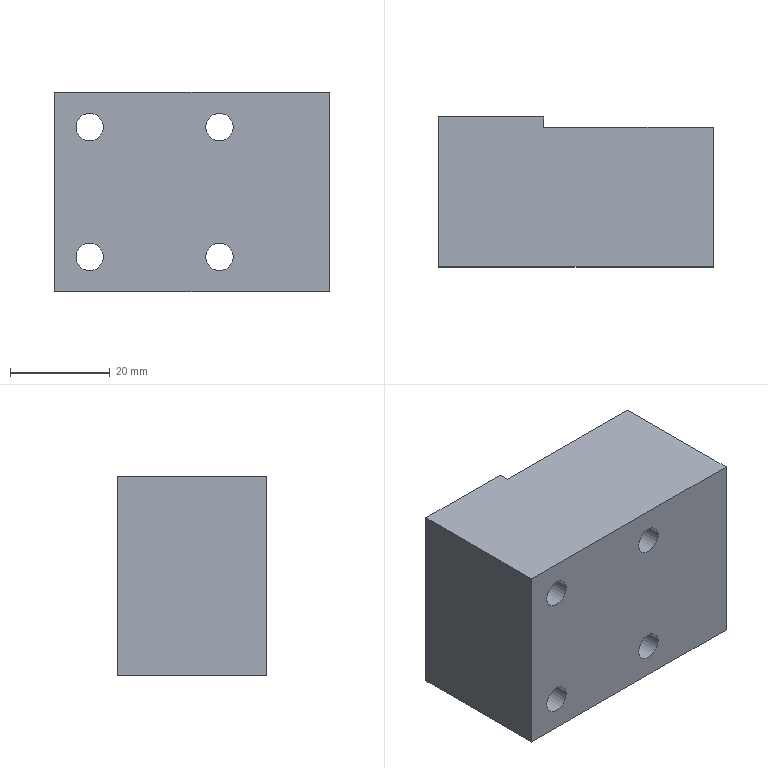Part | NX | features BREP 1 | 1 solid | 24 faces | box 55 x 30 x 40 mm | volume 57495 mm3 | plane 12 | cylinder 10 | cone 2 | commonest cylinder face diameters 5.5 x4 10 x4 6.8 x2
STEP:
#1=CARTESIAN_POINT('',(7.,30.,18.));
#2=VERTEX_POINT('',#1);
#3=CARTESIAN_POINT('',(7.,30.,13.));
#4=DIRECTION('',(0.,1.,0.));
#5=DIRECTION('',(0.,0.,1.));
#6=AXIS2_PLACEMENT_3D('',#3,#4,#5);
#7=CIRCLE('',#6,5.);
#8=EDGE_CURVE('',#2,#2,#7,.T.);
#9=ORIENTED_EDGE('',*,*,#8,.F.);
#10=EDGE_LOOP('',(#9));
#11=FACE_BOUND('',#10,.T.);
#12=CARTESIAN_POINT('',(7.,30.,-8.));
#13=VERTEX_POINT('',#12);
#14=CARTESIAN_POINT('',(7.,30.,-13.));
#15=DIRECTION('',(0.,1.,0.));
#16=DIRECTION('',(0.,0.,1.));
#17=AXIS2_PLACEMENT_3D('',#14,#15,#16);
#18=CIRCLE('',#17,5.);
#19=EDGE_CURVE('',#13,#13,#18,.T.);
#20=ORIENTED_EDGE('',*,*,#19,.F.);
#21=EDGE_LOOP('',(#20));
#22=FACE_BOUND('',#21,.T.);
#23=CARTESIAN_POINT('',(21.,30.,-20.));
#24=VERTEX_POINT('',#23);
#25=CARTESIAN_POINT('',(0.,30.,-20.));
#26=VERTEX_POINT('',#25);
#27=CARTESIAN_POINT('',(21.,30.,-20.));
#28=DIRECTION('',(-1.,0.,0.));
#29=VECTOR('',#28,1000.);
#30=LINE('',#27,#29);
#31=EDGE_CURVE('',#24,#26,#30,.T.);
#32=ORIENTED_EDGE('',*,*,#31,.T.);
#33=CARTESIAN_POINT('',(0.,30.,20.));
#34=VERTEX_POINT('',#33);
#35=CARTESIAN_POINT('',(0.,30.,20.));
#36=DIRECTION('',(0.,0.,-1.));
#37=VECTOR('',#36,1000.);
#38=LINE('',#35,#37);
#39=EDGE_CURVE('',#34,#26,#38,.T.);
#40=ORIENTED_EDGE('',*,*,#39,.F.);
#41=CARTESIAN_POINT('',(21.,30.,20.));
#42=VERTEX_POINT('',#41);
#43=CARTESIAN_POINT('',(21.,30.,20.));
#44=DIRECTION('',(-1.,0.,0.));
#45=VECTOR('',#44,1000.);
#46=LINE('',#43,#45);
#47=EDGE_CURVE('',#42,#34,#46,.T.);
#48=ORIENTED_EDGE('',*,*,#47,.F.);
#49=CARTESIAN_POINT('',(21.,30.,20.));
#50=DIRECTION('',(0.,0.,-1.));
#51=VECTOR('',#50,1000.);
#52=LINE('',#49,#51);
#53=EDGE_CURVE('',#42,#24,#52,.T.);
#54=ORIENTED_EDGE('',*,*,#53,.T.);
#55=EDGE_LOOP('',(#32,#40,#48,#54));
#56=FACE_BOUND('',#55,.T.);
#57=CARTESIAN_POINT('',(21.,30.,20.));
#58=DIRECTION('',(0.,-1.,0.));
#59=DIRECTION('',(0.,0.,1.));
#60=AXIS2_PLACEMENT_3D('',#57,#58,#59);
#61=PLANE('',#60);
#62=ADVANCED_FACE('',(#11,#22,#56),#61,.F.);
#63=CARTESIAN_POINT('',(0.,0.,-20.));
#64=VERTEX_POINT('',#63);
#65=CARTESIAN_POINT('',(0.,30.,-20.));
#66=DIRECTION('',(0.,-1.,0.));
#67=VECTOR('',#66,1000.);
#68=LINE('',#65,#67);
#69=EDGE_CURVE('',#26,#64,#68,.T.);
#70=ORIENTED_EDGE('',*,*,#69,.T.);
#71=CARTESIAN_POINT('',(0.,0.,20.));
#72=VERTEX_POINT('',#71);
#73=CARTESIAN_POINT('',(0.,0.,20.));
#74=DIRECTION('',(0.,0.,-1.));
#75=VECTOR('',#74,1000.);
#76=LINE('',#73,#75);
#77=EDGE_CURVE('',#72,#64,#76,.T.);
#78=ORIENTED_EDGE('',*,*,#77,.F.);
#79=CARTESIAN_POINT('',(0.,30.,20.));
#80=DIRECTION('',(0.,-1.,0.));
#81=VECTOR('',#80,1000.);
#82=LINE('',#79,#81);
#83=EDGE_CURVE('',#34,#72,#82,.T.);
#84=ORIENTED_EDGE('',*,*,#83,.F.);
#85=ORIENTED_EDGE('',*,*,#39,.T.);
#86=EDGE_LOOP('',(#70,#78,#84,#85));
#87=FACE_BOUND('',#86,.T.);
#88=CARTESIAN_POINT('',(0.,30.,20.));
#89=DIRECTION('',(1.,0.,0.));
#90=DIRECTION('',(0.,-1.,0.));
#91=AXIS2_PLACEMENT_3D('',#88,#89,#90);
#92=PLANE('',#91);
#93=ADVANCED_FACE('',(#87),#92,.F.);
#94=CARTESIAN_POINT('',(33.,0.,-10.25));
#95=VERTEX_POINT('',#94);
#96=CARTESIAN_POINT('',(33.,0.,-13.));
#97=DIRECTION('',(0.,1.,0.));
#98=DIRECTION('',(0.,0.,1.));
#99=AXIS2_PLACEMENT_3D('',#96,#97,#98);
#100=CIRCLE('',#99,2.75);
#101=EDGE_CURVE('',#95,#95,#100,.T.);
#102=ORIENTED_EDGE('',*,*,#101,.T.);
#103=EDGE_LOOP('',(#102));
#104=FACE_BOUND('',#103,.T.);
#105=CARTESIAN_POINT('',(7.,0.,15.75));
#106=VERTEX_POINT('',#105);
#107=CARTESIAN_POINT('',(7.,0.,13.));
#108=DIRECTION('',(0.,1.,0.));
#109=DIRECTION('',(0.,0.,1.));
#110=AXIS2_PLACEMENT_3D('',#107,#108,#109);
#111=CIRCLE('',#110,2.75);
#112=EDGE_CURVE('',#106,#106,#111,.T.);
#113=ORIENTED_EDGE('',*,*,#112,.T.);
#114=EDGE_LOOP('',(#113));
#115=FACE_BOUND('',#114,.T.);
#116=CARTESIAN_POINT('',(33.,0.,15.75));
#117=VERTEX_POINT('',#116);
#118=CARTESIAN_POINT('',(33.,0.,13.));
#119=DIRECTION('',(0.,1.,0.));
#120=DIRECTION('',(0.,0.,1.));
#121=AXIS2_PLACEMENT_3D('',#118,#119,#120);
#122=CIRCLE('',#121,2.75);
#123=EDGE_CURVE('',#117,#117,#122,.T.);
#124=ORIENTED_EDGE('',*,*,#123,.T.);
#125=EDGE_LOOP('',(#124));
#126=FACE_BOUND('',#125,.T.);
#127=CARTESIAN_POINT('',(7.,0.,-10.25));
#128=VERTEX_POINT('',#127);
#129=CARTESIAN_POINT('',(7.,0.,-13.));
#130=DIRECTION('',(0.,1.,0.));
#131=DIRECTION('',(0.,0.,1.));
#132=AXIS2_PLACEMENT_3D('',#129,#130,#131);
#133=CIRCLE('',#132,2.75);
#134=EDGE_CURVE('',#128,#128,#133,.T.);
#135=ORIENTED_EDGE('',*,*,#134,.T.);
#136=EDGE_LOOP('',(#135));
#137=FACE_BOUND('',#136,.T.);
#138=CARTESIAN_POINT('',(55.,0.,-20.));
#139=VERTEX_POINT('',#138);
#140=CARTESIAN_POINT('',(0.,0.,-20.));
#141=DIRECTION('',(1.,0.,0.));
#142=VECTOR('',#141,1000.);
#143=LINE('',#140,#142);
#144=EDGE_CURVE('',#64,#139,#143,.T.);
#145=ORIENTED_EDGE('',*,*,#144,.T.);
#146=CARTESIAN_POINT('',(55.,0.,20.));
#147=VERTEX_POINT('',#146);
#148=CARTESIAN_POINT('',(55.,0.,20.));
#149=DIRECTION('',(0.,0.,-1.));
#150=VECTOR('',#149,1000.);
#151=LINE('',#148,#150);
#152=EDGE_CURVE('',#147,#139,#151,.T.);
#153=ORIENTED_EDGE('',*,*,#152,.F.);
#154=CARTESIAN_POINT('',(0.,0.,20.));
#155=DIRECTION('',(1.,0.,0.));
#156=VECTOR('',#155,1000.);
#157=LINE('',#154,#156);
#158=EDGE_CURVE('',#72,#147,#157,.T.);
#159=ORIENTED_EDGE('',*,*,#158,.F.);
#160=ORIENTED_EDGE('',*,*,#77,.T.);
#161=EDGE_LOOP('',(#145,#153,#159,#160));
#162=FACE_BOUND('',#161,.T.);
#163=CARTESIAN_POINT('',(0.,0.,20.));
#164=DIRECTION('',(0.,1.,0.));
#165=DIRECTION('',(0.,0.,-1.));
#166=AXIS2_PLACEMENT_3D('',#163,#164,#165);
#167=PLANE('',#166);
#168=ADVANCED_FACE('',(#104,#115,#126,#137,#162),#167,.F.);
#169=CARTESIAN_POINT('',(55.,27.9,-20.));
#170=VERTEX_POINT('',#169);
#171=CARTESIAN_POINT('',(55.,0.,-20.));
#172=DIRECTION('',(0.,1.,0.));
#173=VECTOR('',#172,1000.);
#174=LINE('',#171,#173);
#175=EDGE_CURVE('',#139,#170,#174,.T.);
#176=ORIENTED_EDGE('',*,*,#175,.T.);
#177=CARTESIAN_POINT('',(55.,27.9,20.));
#178=VERTEX_POINT('',#177);
#179=CARTESIAN_POINT('',(55.,27.9,20.));
#180=DIRECTION('',(0.,0.,-1.));
#181=VECTOR('',#180,1000.);
#182=LINE('',#179,#181);
#183=EDGE_CURVE('',#178,#170,#182,.T.);
#184=ORIENTED_EDGE('',*,*,#183,.F.);
#185=CARTESIAN_POINT('',(55.,0.,20.));
#186=DIRECTION('',(0.,1.,0.));
#187=VECTOR('',#186,1000.);
#188=LINE('',#185,#187);
#189=EDGE_CURVE('',#147,#178,#188,.T.);
#190=ORIENTED_EDGE('',*,*,#189,.F.);
#191=ORIENTED_EDGE('',*,*,#152,.T.);
#192=EDGE_LOOP('',(#176,#184,#190,#191));
#193=FACE_BOUND('',#192,.T.);
#194=CARTESIAN_POINT('',(55.,0.,20.));
#195=DIRECTION('',(-1.,0.,0.));
#196=DIRECTION('',(0.,0.,-1.));
#197=AXIS2_PLACEMENT_3D('',#194,#195,#196);
#198=PLANE('',#197);
#199=ADVANCED_FACE('',(#193),#198,.F.);
#200=CARTESIAN_POINT('',(33.,27.9,-8.));
#201=VERTEX_POINT('',#200);
#202=CARTESIAN_POINT('',(33.,27.9,-13.));
#203=DIRECTION('',(0.,1.,0.));
#204=DIRECTION('',(0.,0.,1.));
#205=AXIS2_PLACEMENT_3D('',#202,#203,#204);
#206=CIRCLE('',#205,5.);
#207=EDGE_CURVE('',#201,#201,#206,.T.);
#208=ORIENTED_EDGE('',*,*,#207,.F.);
#209=EDGE_LOOP('',(#208));
#210=FACE_BOUND('',#209,.T.);
#211=CARTESIAN_POINT('',(33.,27.9,18.));
#212=VERTEX_POINT('',#211);
#213=CARTESIAN_POINT('',(33.,27.9,13.));
#214=DIRECTION('',(0.,1.,0.));
#215=DIRECTION('',(0.,0.,1.));
#216=AXIS2_PLACEMENT_3D('',#213,#214,#215);
#217=CIRCLE('',#216,5.);
#218=EDGE_CURVE('',#212,#212,#217,.T.);
#219=ORIENTED_EDGE('',*,*,#218,.F.);
#220=EDGE_LOOP('',(#219));
#221=FACE_BOUND('',#220,.T.);
#222=CARTESIAN_POINT('',(29.,27.9,0.4));
#223=VERTEX_POINT('',#222);
#224=CARTESIAN_POINT('',(29.,27.9,-3.));
#225=DIRECTION('',(0.,1.,0.));
#226=DIRECTION('',(0.,0.,1.));
#227=AXIS2_PLACEMENT_3D('',#224,#225,#226);
#228=CIRCLE('',#227,3.4);
#229=EDGE_CURVE('',#223,#223,#228,.T.);
#230=ORIENTED_EDGE('',*,*,#229,.F.);
#231=EDGE_LOOP('',(#230));
#232=FACE_BOUND('',#231,.T.);
#233=CARTESIAN_POINT('',(45.,27.9,0.4));
#234=VERTEX_POINT('',#233);
#235=CARTESIAN_POINT('',(45.,27.9,-3.));
#236=DIRECTION('',(0.,1.,0.));
#237=DIRECTION('',(0.,0.,1.));
#238=AXIS2_PLACEMENT_3D('',#235,#236,#237);
#239=CIRCLE('',#238,3.4);
#240=EDGE_CURVE('',#234,#234,#239,.T.);
#241=ORIENTED_EDGE('',*,*,#240,.F.);
#242=EDGE_LOOP('',(#241));
#243=FACE_BOUND('',#242,.T.);
#244=CARTESIAN_POINT('',(21.,27.9,-20.));
#245=VERTEX_POINT('',#244);
#246=CARTESIAN_POINT('',(55.,27.9,-20.));
#247=DIRECTION('',(-1.,0.,0.));
#248=VECTOR('',#247,1000.);
#249=LINE('',#246,#248);
#250=EDGE_CURVE('',#170,#245,#249,.T.);
#251=ORIENTED_EDGE('',*,*,#250,.T.);
#252=CARTESIAN_POINT('',(21.,27.9,20.));
#253=VERTEX_POINT('',#252);
#254=CARTESIAN_POINT('',(21.,27.9,20.));
#255=DIRECTION('',(0.,0.,-1.));
#256=VECTOR('',#255,1000.);
#257=LINE('',#254,#256);
#258=EDGE_CURVE('',#253,#245,#257,.T.);
#259=ORIENTED_EDGE('',*,*,#258,.F.);
#260=CARTESIAN_POINT('',(55.,27.9,20.));
#261=DIRECTION('',(-1.,0.,0.));
#262=VECTOR('',#261,1000.);
#263=LINE('',#260,#262);
#264=EDGE_CURVE('',#178,#253,#263,.T.);
#265=ORIENTED_EDGE('',*,*,#264,.F.);
#266=ORIENTED_EDGE('',*,*,#183,.T.);
#267=EDGE_LOOP('',(#251,#259,#265,#266));
#268=FACE_BOUND('',#267,.T.);
#269=CARTESIAN_POINT('',(55.,27.9,20.));
#270=DIRECTION('',(0.,-1.,0.));
#271=DIRECTION('',(-1.,0.,0.));
#272=AXIS2_PLACEMENT_3D('',#269,#270,#271);
#273=PLANE('',#272);
#274=ADVANCED_FACE('',(#210,#221,#232,#243,#268),#273,.F.);
#275=CARTESIAN_POINT('',(21.,27.9,-20.));
#276=DIRECTION('',(0.,1.,0.));
#277=VECTOR('',#276,1000.);
#278=LINE('',#275,#277);
#279=EDGE_CURVE('',#245,#24,#278,.T.);
#280=ORIENTED_EDGE('',*,*,#279,.T.);
#281=ORIENTED_EDGE('',*,*,#53,.F.);
#282=CARTESIAN_POINT('',(21.,27.9,20.));
#283=DIRECTION('',(0.,1.,0.));
#284=VECTOR('',#283,1000.);
#285=LINE('',#282,#284);
#286=EDGE_CURVE('',#253,#42,#285,.T.);
#287=ORIENTED_EDGE('',*,*,#286,.F.);
#288=ORIENTED_EDGE('',*,*,#258,.T.);
#289=EDGE_LOOP('',(#280,#281,#287,#288));
#290=FACE_BOUND('',#289,.T.);
#291=CARTESIAN_POINT('',(21.,27.9,20.));
#292=DIRECTION('',(-1.,0.,0.));
#293=DIRECTION('',(0.,1.,0.));
#294=AXIS2_PLACEMENT_3D('',#291,#292,#293);
#295=PLANE('',#294);
#296=ADVANCED_FACE('',(#290),#295,.F.);
#297=ORIENTED_EDGE('',*,*,#47,.T.);
#298=ORIENTED_EDGE('',*,*,#83,.T.);
#299=ORIENTED_EDGE('',*,*,#158,.T.);
#300=ORIENTED_EDGE('',*,*,#189,.T.);
#301=ORIENTED_EDGE('',*,*,#264,.T.);
#302=ORIENTED_EDGE('',*,*,#286,.T.);
#303=EDGE_LOOP('',(#297,#298,#299,#300,#301,#302));
#304=FACE_BOUND('',#303,.T.);
#305=CARTESIAN_POINT('',(0.,0.,20.));
#306=DIRECTION('',(0.,0.,1.));
#307=DIRECTION('',(-1.,0.,0.));
#308=AXIS2_PLACEMENT_3D('',#305,#306,#307);
#309=PLANE('',#308);
#310=ADVANCED_FACE('',(#304),#309,.T.);
#311=ORIENTED_EDGE('',*,*,#31,.F.);
#312=ORIENTED_EDGE('',*,*,#279,.F.);
#313=ORIENTED_EDGE('',*,*,#250,.F.);
#314=ORIENTED_EDGE('',*,*,#175,.F.);
#315=ORIENTED_EDGE('',*,*,#144,.F.);
#316=ORIENTED_EDGE('',*,*,#69,.F.);
#317=EDGE_LOOP('',(#311,#312,#313,#314,#315,#316));
#318=FACE_BOUND('',#317,.T.);
#319=CARTESIAN_POINT('',(0.,0.,-20.));
#320=DIRECTION('',(0.,0.,1.));
#321=DIRECTION('',(-1.,0.,0.));
#322=AXIS2_PLACEMENT_3D('',#319,#320,#321);
#323=PLANE('',#322);
#324=ADVANCED_FACE('',(#318),#323,.F.);
#325=CARTESIAN_POINT('',(45.,6.107,-3.));
#326=VERTEX_POINT('',#325);
#327=VERTEX_LOOP('',#326);
#328=FACE_BOUND('',#327,.T.);
#329=CARTESIAN_POINT('',(45.,8.15,0.4));
#330=VERTEX_POINT('',#329);
#331=CARTESIAN_POINT('',(45.,8.15,-3.));
#332=DIRECTION('',(0.,1.,0.));
#333=DIRECTION('',(0.,0.,1.));
#334=AXIS2_PLACEMENT_3D('',#331,#332,#333);
#335=CIRCLE('',#334,3.4);
#336=EDGE_CURVE('',#330,#330,#335,.T.);
#337=ORIENTED_EDGE('',*,*,#336,.T.);
#338=EDGE_LOOP('',(#337));
#339=FACE_BOUND('',#338,.T.);
#340=CARTESIAN_POINT('',(45.,8.15,-3.));
#341=DIRECTION('',(0.,1.,0.));
#342=DIRECTION('',(0.,0.,-1.));
#343=AXIS2_PLACEMENT_3D('',#340,#341,#342);
#344=CONICAL_SURFACE('',#343,3.4,1.03);
#345=ADVANCED_FACE('',(#328,#339),#344,.F.);
#346=ORIENTED_EDGE('',*,*,#336,.F.);
#347=EDGE_LOOP('',(#346));
#348=FACE_BOUND('',#347,.T.);
#349=ORIENTED_EDGE('',*,*,#240,.T.);
#350=EDGE_LOOP('',(#349));
#351=FACE_BOUND('',#350,.T.);
#352=CARTESIAN_POINT('',(45.,27.9,-3.));
#353=DIRECTION('',(0.,1.,0.));
#354=DIRECTION('',(0.,0.,-1.));
#355=AXIS2_PLACEMENT_3D('',#352,#353,#354);
#356=CYLINDRICAL_SURFACE('',#355,3.4);
#357=ADVANCED_FACE('',(#348,#351),#356,.F.);
#358=CARTESIAN_POINT('',(29.,6.107,-3.));
#359=VERTEX_POINT('',#358);
#360=VERTEX_LOOP('',#359);
#361=FACE_BOUND('',#360,.T.);
#362=CARTESIAN_POINT('',(29.,8.15,0.4));
#363=VERTEX_POINT('',#362);
#364=CARTESIAN_POINT('',(29.,8.15,-3.));
#365=DIRECTION('',(0.,1.,0.));
#366=DIRECTION('',(0.,0.,1.));
#367=AXIS2_PLACEMENT_3D('',#364,#365,#366);
#368=CIRCLE('',#367,3.4);
#369=EDGE_CURVE('',#363,#363,#368,.T.);
#370=ORIENTED_EDGE('',*,*,#369,.T.);
#371=EDGE_LOOP('',(#370));
#372=FACE_BOUND('',#371,.T.);
#373=CARTESIAN_POINT('',(29.,8.15,-3.));
#374=DIRECTION('',(0.,1.,0.));
#375=DIRECTION('',(0.,0.,-1.));
#376=AXIS2_PLACEMENT_3D('',#373,#374,#375);
#377=CONICAL_SURFACE('',#376,3.4,1.03);
#378=ADVANCED_FACE('',(#361,#372),#377,.F.);
#379=ORIENTED_EDGE('',*,*,#369,.F.);
#380=EDGE_LOOP('',(#379));
#381=FACE_BOUND('',#380,.T.);
#382=ORIENTED_EDGE('',*,*,#229,.T.);
#383=EDGE_LOOP('',(#382));
#384=FACE_BOUND('',#383,.T.);
#385=CARTESIAN_POINT('',(29.,27.9,-3.));
#386=DIRECTION('',(0.,1.,0.));
#387=DIRECTION('',(0.,0.,-1.));
#388=AXIS2_PLACEMENT_3D('',#385,#386,#387);
#389=CYLINDRICAL_SURFACE('',#388,3.4);
#390=ADVANCED_FACE('',(#381,#384),#389,.F.);
#391=ORIENTED_EDGE('',*,*,#134,.F.);
#392=EDGE_LOOP('',(#391));
#393=FACE_BOUND('',#392,.T.);
#394=CARTESIAN_POINT('',(7.,22.5,-10.25));
#395=VERTEX_POINT('',#394);
#396=CARTESIAN_POINT('',(7.,22.5,-13.));
#397=DIRECTION('',(0.,1.,0.));
#398=DIRECTION('',(0.,0.,1.));
#399=AXIS2_PLACEMENT_3D('',#396,#397,#398);
#400=CIRCLE('',#399,2.75);
#401=EDGE_CURVE('',#395,#395,#400,.T.);
#402=ORIENTED_EDGE('',*,*,#401,.T.);
#403=EDGE_LOOP('',(#402));
#404=FACE_BOUND('',#403,.T.);
#405=CARTESIAN_POINT('',(7.,27.9,-13.));
#406=DIRECTION('',(0.,1.,0.));
#407=DIRECTION('',(0.,0.,-1.));
#408=AXIS2_PLACEMENT_3D('',#405,#406,#407);
#409=CYLINDRICAL_SURFACE('',#408,2.75);
#410=ADVANCED_FACE('',(#393,#404),#409,.F.);
#411=ORIENTED_EDGE('',*,*,#401,.F.);
#412=EDGE_LOOP('',(#411));
#413=FACE_BOUND('',#412,.T.);
#414=CARTESIAN_POINT('',(7.,22.5,-8.));
#415=VERTEX_POINT('',#414);
#416=CARTESIAN_POINT('',(7.,22.5,-13.));
#417=DIRECTION('',(0.,1.,0.));
#418=DIRECTION('',(0.,0.,1.));
#419=AXIS2_PLACEMENT_3D('',#416,#417,#418);
#420=CIRCLE('',#419,5.);
#421=EDGE_CURVE('',#415,#415,#420,.T.);
#422=ORIENTED_EDGE('',*,*,#421,.T.);
#423=EDGE_LOOP('',(#422));
#424=FACE_BOUND('',#423,.T.);
#425=CARTESIAN_POINT('',(9.75,22.5,-13.));
#426=DIRECTION('',(0.,-1.,0.));
#427=DIRECTION('',(0.,0.,1.));
#428=AXIS2_PLACEMENT_3D('',#425,#426,#427);
#429=PLANE('',#428);
#430=ADVANCED_FACE('',(#413,#424),#429,.F.);
#431=ORIENTED_EDGE('',*,*,#421,.F.);
#432=EDGE_LOOP('',(#431));
#433=FACE_BOUND('',#432,.T.);
#434=ORIENTED_EDGE('',*,*,#19,.T.);
#435=EDGE_LOOP('',(#434));
#436=FACE_BOUND('',#435,.T.);
#437=CARTESIAN_POINT('',(7.,27.9,-13.));
#438=DIRECTION('',(0.,1.,0.));
#439=DIRECTION('',(0.,0.,-1.));
#440=AXIS2_PLACEMENT_3D('',#437,#438,#439);
#441=CYLINDRICAL_SURFACE('',#440,5.);
#442=ADVANCED_FACE('',(#433,#436),#441,.F.);
#443=ORIENTED_EDGE('',*,*,#123,.F.);
#444=EDGE_LOOP('',(#443));
#445=FACE_BOUND('',#444,.T.);
#446=CARTESIAN_POINT('',(33.,22.5,15.75));
#447=VERTEX_POINT('',#446);
#448=CARTESIAN_POINT('',(33.,22.5,13.));
#449=DIRECTION('',(0.,1.,0.));
#450=DIRECTION('',(0.,0.,1.));
#451=AXIS2_PLACEMENT_3D('',#448,#449,#450);
#452=CIRCLE('',#451,2.75);
#453=EDGE_CURVE('',#447,#447,#452,.T.);
#454=ORIENTED_EDGE('',*,*,#453,.T.);
#455=EDGE_LOOP('',(#454));
#456=FACE_BOUND('',#455,.T.);
#457=CARTESIAN_POINT('',(33.,27.9,13.));
#458=DIRECTION('',(0.,1.,0.));
#459=DIRECTION('',(0.,0.,-1.));
#460=AXIS2_PLACEMENT_3D('',#457,#458,#459);
#461=CYLINDRICAL_SURFACE('',#460,2.75);
#462=ADVANCED_FACE('',(#445,#456),#461,.F.);
#463=ORIENTED_EDGE('',*,*,#453,.F.);
#464=EDGE_LOOP('',(#463));
#465=FACE_BOUND('',#464,.T.);
#466=CARTESIAN_POINT('',(33.,22.5,18.));
#467=VERTEX_POINT('',#466);
#468=CARTESIAN_POINT('',(33.,22.5,13.));
#469=DIRECTION('',(0.,1.,0.));
#470=DIRECTION('',(0.,0.,1.));
#471=AXIS2_PLACEMENT_3D('',#468,#469,#470);
#472=CIRCLE('',#471,5.);
#473=EDGE_CURVE('',#467,#467,#472,.T.);
#474=ORIENTED_EDGE('',*,*,#473,.T.);
#475=EDGE_LOOP('',(#474));
#476=FACE_BOUND('',#475,.T.);
#477=CARTESIAN_POINT('',(35.75,22.5,13.));
#478=DIRECTION('',(0.,-1.,0.));
#479=DIRECTION('',(0.,0.,1.));
#480=AXIS2_PLACEMENT_3D('',#477,#478,#479);
#481=PLANE('',#480);
#482=ADVANCED_FACE('',(#465,#476),#481,.F.);
#483=ORIENTED_EDGE('',*,*,#473,.F.);
#484=EDGE_LOOP('',(#483));
#485=FACE_BOUND('',#484,.T.);
#486=ORIENTED_EDGE('',*,*,#218,.T.);
#487=EDGE_LOOP('',(#486));
#488=FACE_BOUND('',#487,.T.);
#489=CARTESIAN_POINT('',(33.,27.9,13.));
#490=DIRECTION('',(0.,1.,0.));
#491=DIRECTION('',(0.,0.,-1.));
#492=AXIS2_PLACEMENT_3D('',#489,#490,#491);
#493=CYLINDRICAL_SURFACE('',#492,5.);
#494=ADVANCED_FACE('',(#485,#488),#493,.F.);
#495=ORIENTED_EDGE('',*,*,#112,.F.);
#496=EDGE_LOOP('',(#495));
#497=FACE_BOUND('',#496,.T.);
#498=CARTESIAN_POINT('',(7.,22.5,15.75));
#499=VERTEX_POINT('',#498);
#500=CARTESIAN_POINT('',(7.,22.5,13.));
#501=DIRECTION('',(0.,1.,0.));
#502=DIRECTION('',(0.,0.,1.));
#503=AXIS2_PLACEMENT_3D('',#500,#501,#502);
#504=CIRCLE('',#503,2.75);
#505=EDGE_CURVE('',#499,#499,#504,.T.);
#506=ORIENTED_EDGE('',*,*,#505,.T.);
#507=EDGE_LOOP('',(#506));
#508=FACE_BOUND('',#507,.T.);
#509=CARTESIAN_POINT('',(7.,27.9,13.));
#510=DIRECTION('',(0.,1.,0.));
#511=DIRECTION('',(0.,0.,-1.));
#512=AXIS2_PLACEMENT_3D('',#509,#510,#511);
#513=CYLINDRICAL_SURFACE('',#512,2.75);
#514=ADVANCED_FACE('',(#497,#508),#513,.F.);
#515=ORIENTED_EDGE('',*,*,#505,.F.);
#516=EDGE_LOOP('',(#515));
#517=FACE_BOUND('',#516,.T.);
#518=CARTESIAN_POINT('',(7.,22.5,18.));
#519=VERTEX_POINT('',#518);
#520=CARTESIAN_POINT('',(7.,22.5,13.));
#521=DIRECTION('',(0.,1.,0.));
#522=DIRECTION('',(0.,0.,1.));
#523=AXIS2_PLACEMENT_3D('',#520,#521,#522);
#524=CIRCLE('',#523,5.);
#525=EDGE_CURVE('',#519,#519,#524,.T.);
#526=ORIENTED_EDGE('',*,*,#525,.T.);
#527=EDGE_LOOP('',(#526));
#528=FACE_BOUND('',#527,.T.);
#529=CARTESIAN_POINT('',(9.75,22.5,13.));
#530=DIRECTION('',(0.,-1.,0.));
#531=DIRECTION('',(0.,0.,1.));
#532=AXIS2_PLACEMENT_3D('',#529,#530,#531);
#533=PLANE('',#532);
#534=ADVANCED_FACE('',(#517,#528),#533,.F.);
#535=ORIENTED_EDGE('',*,*,#525,.F.);
#536=EDGE_LOOP('',(#535));
#537=FACE_BOUND('',#536,.T.);
#538=ORIENTED_EDGE('',*,*,#8,.T.);
#539=EDGE_LOOP('',(#538));
#540=FACE_BOUND('',#539,.T.);
#541=CARTESIAN_POINT('',(7.,27.9,13.));
#542=DIRECTION('',(0.,1.,0.));
#543=DIRECTION('',(0.,0.,-1.));
#544=AXIS2_PLACEMENT_3D('',#541,#542,#543);
#545=CYLINDRICAL_SURFACE('',#544,5.);
#546=ADVANCED_FACE('',(#537,#540),#545,.F.);
#547=ORIENTED_EDGE('',*,*,#101,.F.);
#548=EDGE_LOOP('',(#547));
#549=FACE_BOUND('',#548,.T.);
#550=CARTESIAN_POINT('',(33.,22.5,-10.25));
#551=VERTEX_POINT('',#550);
#552=CARTESIAN_POINT('',(33.,22.5,-13.));
#553=DIRECTION('',(0.,1.,0.));
#554=DIRECTION('',(0.,0.,1.));
#555=AXIS2_PLACEMENT_3D('',#552,#553,#554);
#556=CIRCLE('',#555,2.75);
#557=EDGE_CURVE('',#551,#551,#556,.T.);
#558=ORIENTED_EDGE('',*,*,#557,.T.);
#559=EDGE_LOOP('',(#558));
#560=FACE_BOUND('',#559,.T.);
#561=CARTESIAN_POINT('',(33.,27.9,-13.));
#562=DIRECTION('',(0.,1.,0.));
#563=DIRECTION('',(0.,0.,-1.));
#564=AXIS2_PLACEMENT_3D('',#561,#562,#563);
#565=CYLINDRICAL_SURFACE('',#564,2.75);
#566=ADVANCED_FACE('',(#549,#560),#565,.F.);
#567=ORIENTED_EDGE('',*,*,#557,.F.);
#568=EDGE_LOOP('',(#567));
#569=FACE_BOUND('',#568,.T.);
#570=CARTESIAN_POINT('',(33.,22.5,-8.));
#571=VERTEX_POINT('',#570);
#572=CARTESIAN_POINT('',(33.,22.5,-13.));
#573=DIRECTION('',(0.,1.,0.));
#574=DIRECTION('',(0.,0.,1.));
#575=AXIS2_PLACEMENT_3D('',#572,#573,#574);
#576=CIRCLE('',#575,5.);
#577=EDGE_CURVE('',#571,#571,#576,.T.);
#578=ORIENTED_EDGE('',*,*,#577,.T.);
#579=EDGE_LOOP('',(#578));
#580=FACE_BOUND('',#579,.T.);
#581=CARTESIAN_POINT('',(35.75,22.5,-13.));
#582=DIRECTION('',(0.,-1.,0.));
#583=DIRECTION('',(0.,0.,1.));
#584=AXIS2_PLACEMENT_3D('',#581,#582,#583);
#585=PLANE('',#584);
#586=ADVANCED_FACE('',(#569,#580),#585,.F.);
#587=ORIENTED_EDGE('',*,*,#577,.F.);
#588=EDGE_LOOP('',(#587));
#589=FACE_BOUND('',#588,.T.);
#590=ORIENTED_EDGE('',*,*,#207,.T.);
#591=EDGE_LOOP('',(#590));
#592=FACE_BOUND('',#591,.T.);
#593=CARTESIAN_POINT('',(33.,27.9,-13.));
#594=DIRECTION('',(0.,1.,0.));
#595=DIRECTION('',(0.,0.,-1.));
#596=AXIS2_PLACEMENT_3D('',#593,#594,#595);
#597=CYLINDRICAL_SURFACE('',#596,5.);
#598=ADVANCED_FACE('',(#589,#592),#597,.F.);
#599=CLOSED_SHELL('',(#62,#93,#168,#199,#274,#296,#310,#324,#345,#357,#378,#390,#410,#430,#442,#462,#482,#494,#514,#534,#546,#566,#586,#598));
#600=MANIFOLD_SOLID_BREP('',#599);
#601=(LENGTH_UNIT()NAMED_UNIT(*)SI_UNIT(.MILLI.,.METRE.));
#602=UNCERTAINTY_MEASURE_WITH_UNIT(LENGTH_MEASURE(0.00001),#601,'','');
#603=(NAMED_UNIT(*)PLANE_ANGLE_UNIT()SI_UNIT($,.RADIAN.));
#604=(NAMED_UNIT(*)SI_UNIT($,.STERADIAN.)SOLID_ANGLE_UNIT());
#605=(GEOMETRIC_REPRESENTATION_CONTEXT(3)GLOBAL_UNCERTAINTY_ASSIGNED_CONTEXT((#602))GLOBAL_UNIT_ASSIGNED_CONTEXT((#601,#603,#604))REPRESENTATION_CONTEXT('',''));
#606=ADVANCED_BREP_SHAPE_REPRESENTATION('',(#600),#605);